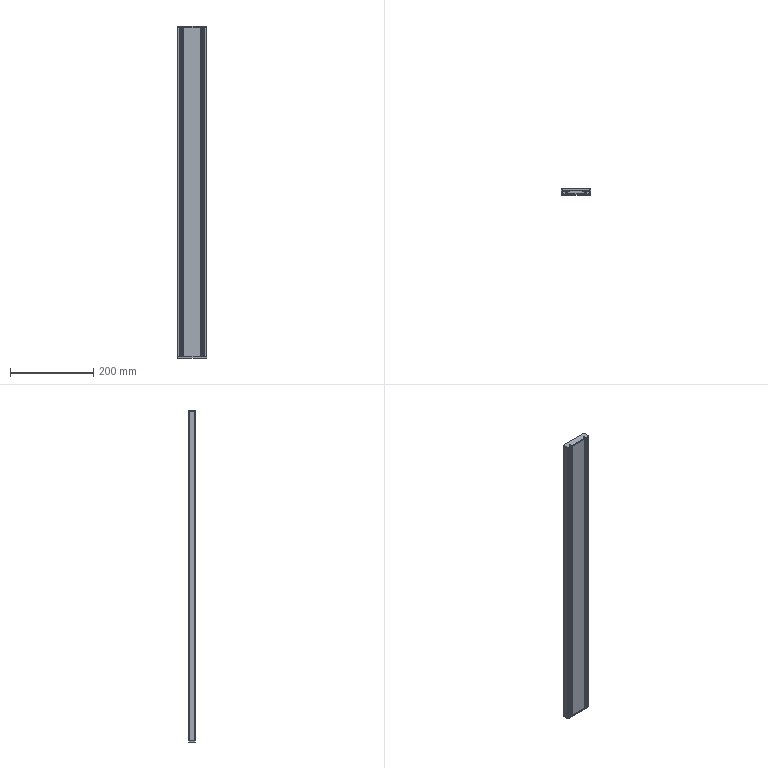Part | 4 solids | 109 faces | box 70 x 15 x 800 mm | volume 506225 mm3 | plane 60 | cylinder 49 | commonest cylinder face diameters 1 x12 2 x12 4 x8 6 x6 0.4 x4 1.1 x4